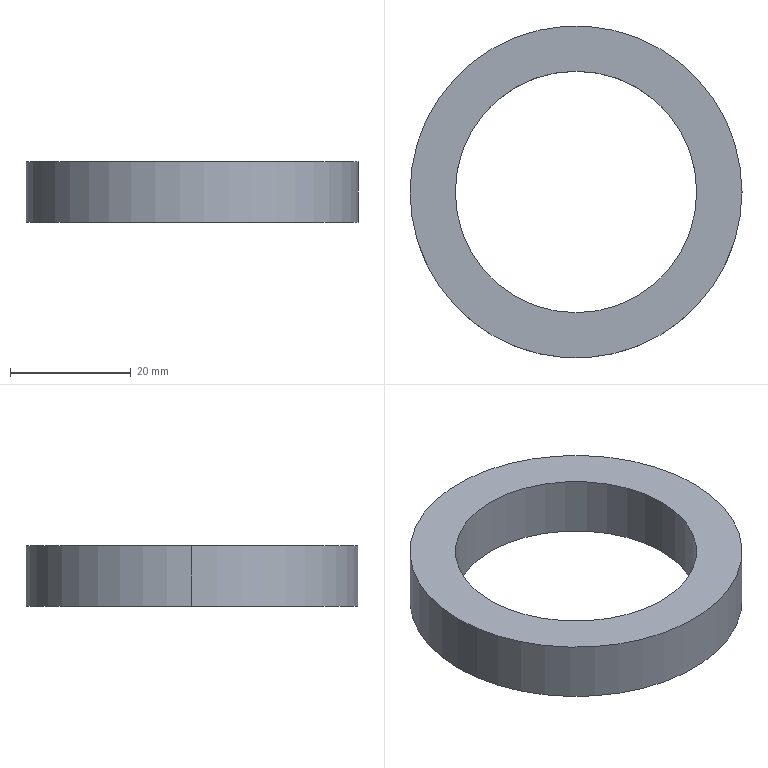Part | SolidWorks | features BaseBody 1 | 1 solid | 6 faces | box 55 x 55 x 10 mm | volume 11192 mm3 | cylinder 4 | plane 2 | commonest cylinder face diameters 40 x2 55 x2
STEP:
#1=CARTESIAN_POINT('',(27.5,0.,0.));
#2=VERTEX_POINT('',#1);
#3=CARTESIAN_POINT('',(-27.5,0.,0.));
#4=VERTEX_POINT('',#3);
#5=CARTESIAN_POINT('',(0.,0.,0.));
#6=DIRECTION('',(0.,0.,1.));
#7=DIRECTION('',(1.,0.,0.));
#8=AXIS2_PLACEMENT_3D('',#5,#6,#7);
#9=CIRCLE('',#8,27.5);
#10=EDGE_CURVE('',#2,#4,#9,.T.);
#11=ORIENTED_EDGE('',*,*,#10,.T.);
#12=CARTESIAN_POINT('',(-27.5,0.,10.));
#13=VERTEX_POINT('',#12);
#14=CARTESIAN_POINT('',(-27.5,0.,0.));
#15=DIRECTION('',(0.,0.,1.));
#16=VECTOR('',#15,1000.);
#17=LINE('',#14,#16);
#18=EDGE_CURVE('',#4,#13,#17,.T.);
#19=ORIENTED_EDGE('',*,*,#18,.T.);
#20=CARTESIAN_POINT('',(27.5,0.,10.));
#21=VERTEX_POINT('',#20);
#22=CARTESIAN_POINT('',(0.,0.,10.));
#23=DIRECTION('',(0.,0.,-1.));
#24=DIRECTION('',(1.,0.,0.));
#25=AXIS2_PLACEMENT_3D('',#22,#23,#24);
#26=CIRCLE('',#25,27.5);
#27=EDGE_CURVE('',#13,#21,#26,.T.);
#28=ORIENTED_EDGE('',*,*,#27,.T.);
#29=CARTESIAN_POINT('',(27.5,0.,0.));
#30=DIRECTION('',(0.,0.,1.));
#31=VECTOR('',#30,1000.);
#32=LINE('',#29,#31);
#33=EDGE_CURVE('',#2,#21,#32,.T.);
#34=ORIENTED_EDGE('',*,*,#33,.F.);
#35=EDGE_LOOP('',(#11,#19,#28,#34));
#36=FACE_OUTER_BOUND('',#35,.T.);
#37=CARTESIAN_POINT('',(0.,0.,0.));
#38=DIRECTION('',(0.,0.,1.));
#39=DIRECTION('',(1.,0.,0.));
#40=AXIS2_PLACEMENT_3D('',#37,#38,#39);
#41=CYLINDRICAL_SURFACE('',#40,27.5);
#42=ADVANCED_FACE('',(#36),#41,.T.);
#43=CARTESIAN_POINT('',(20.,0.,0.));
#44=VERTEX_POINT('',#43);
#45=CARTESIAN_POINT('',(-20.,0.,0.));
#46=VERTEX_POINT('',#45);
#47=CARTESIAN_POINT('',(0.,0.,0.));
#48=DIRECTION('',(0.,0.,-1.));
#49=DIRECTION('',(1.,0.,0.));
#50=AXIS2_PLACEMENT_3D('',#47,#48,#49);
#51=CIRCLE('',#50,20.);
#52=EDGE_CURVE('',#44,#46,#51,.T.);
#53=ORIENTED_EDGE('',*,*,#52,.T.);
#54=CARTESIAN_POINT('',(-20.,0.,10.));
#55=VERTEX_POINT('',#54);
#56=CARTESIAN_POINT('',(-20.,0.,0.));
#57=DIRECTION('',(0.,0.,1.));
#58=VECTOR('',#57,1000.);
#59=LINE('',#56,#58);
#60=EDGE_CURVE('',#46,#55,#59,.T.);
#61=ORIENTED_EDGE('',*,*,#60,.T.);
#62=CARTESIAN_POINT('',(20.,0.,10.));
#63=VERTEX_POINT('',#62);
#64=CARTESIAN_POINT('',(0.,0.,10.));
#65=DIRECTION('',(0.,0.,-1.));
#66=DIRECTION('',(1.,0.,0.));
#67=AXIS2_PLACEMENT_3D('',#64,#65,#66);
#68=CIRCLE('',#67,20.);
#69=EDGE_CURVE('',#63,#55,#68,.T.);
#70=ORIENTED_EDGE('',*,*,#69,.F.);
#71=CARTESIAN_POINT('',(20.,0.,0.));
#72=DIRECTION('',(0.,0.,1.));
#73=VECTOR('',#72,1000.);
#74=LINE('',#71,#73);
#75=EDGE_CURVE('',#44,#63,#74,.T.);
#76=ORIENTED_EDGE('',*,*,#75,.F.);
#77=EDGE_LOOP('',(#53,#61,#70,#76));
#78=FACE_OUTER_BOUND('',#77,.T.);
#79=CARTESIAN_POINT('',(0.,0.,0.));
#80=DIRECTION('',(0.,0.,1.));
#81=DIRECTION('',(1.,0.,0.));
#82=AXIS2_PLACEMENT_3D('',#79,#80,#81);
#83=CYLINDRICAL_SURFACE('',#82,20.);
#84=ADVANCED_FACE('',(#78),#83,.F.);
#85=ORIENTED_EDGE('',*,*,#18,.F.);
#86=CARTESIAN_POINT('',(0.,0.,0.));
#87=DIRECTION('',(0.,0.,1.));
#88=DIRECTION('',(1.,0.,0.));
#89=AXIS2_PLACEMENT_3D('',#86,#87,#88);
#90=CIRCLE('',#89,27.5);
#91=EDGE_CURVE('',#4,#2,#90,.T.);
#92=ORIENTED_EDGE('',*,*,#91,.T.);
#93=ORIENTED_EDGE('',*,*,#33,.T.);
#94=CARTESIAN_POINT('',(0.,0.,10.));
#95=DIRECTION('',(0.,0.,-1.));
#96=DIRECTION('',(1.,0.,0.));
#97=AXIS2_PLACEMENT_3D('',#94,#95,#96);
#98=CIRCLE('',#97,27.5);
#99=EDGE_CURVE('',#21,#13,#98,.T.);
#100=ORIENTED_EDGE('',*,*,#99,.T.);
#101=EDGE_LOOP('',(#85,#92,#93,#100));
#102=FACE_OUTER_BOUND('',#101,.T.);
#103=CARTESIAN_POINT('',(0.,0.,0.));
#104=DIRECTION('',(0.,0.,1.));
#105=DIRECTION('',(1.,0.,0.));
#106=AXIS2_PLACEMENT_3D('',#103,#104,#105);
#107=CYLINDRICAL_SURFACE('',#106,27.5);
#108=ADVANCED_FACE('',(#102),#107,.T.);
#109=ORIENTED_EDGE('',*,*,#52,.F.);
#110=CARTESIAN_POINT('',(0.,0.,0.));
#111=DIRECTION('',(0.,0.,-1.));
#112=DIRECTION('',(1.,0.,0.));
#113=AXIS2_PLACEMENT_3D('',#110,#111,#112);
#114=CIRCLE('',#113,20.);
#115=EDGE_CURVE('',#46,#44,#114,.T.);
#116=ORIENTED_EDGE('',*,*,#115,.F.);
#117=EDGE_LOOP('',(#109,#116));
#118=FACE_BOUND('',#117,.T.);
#119=ORIENTED_EDGE('',*,*,#10,.F.);
#120=ORIENTED_EDGE('',*,*,#91,.F.);
#121=EDGE_LOOP('',(#119,#120));
#122=FACE_OUTER_BOUND('',#121,.T.);
#123=CARTESIAN_POINT('',(0.,0.,0.));
#124=DIRECTION('',(0.,0.,1.));
#125=DIRECTION('',(1.,0.,0.));
#126=AXIS2_PLACEMENT_3D('',#123,#124,#125);
#127=PLANE('',#126);
#128=ADVANCED_FACE('',(#118,#122),#127,.F.);
#129=ORIENTED_EDGE('',*,*,#69,.T.);
#130=CARTESIAN_POINT('',(0.,0.,10.));
#131=DIRECTION('',(0.,0.,-1.));
#132=DIRECTION('',(1.,0.,0.));
#133=AXIS2_PLACEMENT_3D('',#130,#131,#132);
#134=CIRCLE('',#133,20.);
#135=EDGE_CURVE('',#55,#63,#134,.T.);
#136=ORIENTED_EDGE('',*,*,#135,.T.);
#137=EDGE_LOOP('',(#129,#136));
#138=FACE_BOUND('',#137,.T.);
#139=ORIENTED_EDGE('',*,*,#99,.F.);
#140=ORIENTED_EDGE('',*,*,#27,.F.);
#141=EDGE_LOOP('',(#139,#140));
#142=FACE_OUTER_BOUND('',#141,.T.);
#143=CARTESIAN_POINT('',(0.,0.,10.));
#144=DIRECTION('',(0.,0.,1.));
#145=DIRECTION('',(1.,0.,0.));
#146=AXIS2_PLACEMENT_3D('',#143,#144,#145);
#147=PLANE('',#146);
#148=ADVANCED_FACE('',(#138,#142),#147,.T.);
#149=ORIENTED_EDGE('',*,*,#60,.F.);
#150=ORIENTED_EDGE('',*,*,#115,.T.);
#151=ORIENTED_EDGE('',*,*,#75,.T.);
#152=ORIENTED_EDGE('',*,*,#135,.F.);
#153=EDGE_LOOP('',(#149,#150,#151,#152));
#154=FACE_OUTER_BOUND('',#153,.T.);
#155=CARTESIAN_POINT('',(0.,0.,0.));
#156=DIRECTION('',(0.,0.,1.));
#157=DIRECTION('',(1.,0.,0.));
#158=AXIS2_PLACEMENT_3D('',#155,#156,#157);
#159=CYLINDRICAL_SURFACE('',#158,20.);
#160=ADVANCED_FACE('',(#154),#159,.F.);
#161=CLOSED_SHELL('',(#42,#84,#108,#128,#148,#160));
#162=MANIFOLD_SOLID_BREP('',#161);
#163=CARTESIAN_POINT('',(0.,0.,0.));
#164=DIRECTION('',(0.,0.,1.));
#165=DIRECTION('',(1.,0.,0.));
#166=AXIS2_PLACEMENT_3D('',#163,#164,#165);
#167=(LENGTH_UNIT()NAMED_UNIT(*)SI_UNIT(.MILLI.,.METRE.));
#168=UNCERTAINTY_MEASURE_WITH_UNIT(LENGTH_MEASURE(0.00001),#167,'','');
#169=(NAMED_UNIT(*)PLANE_ANGLE_UNIT()SI_UNIT($,.RADIAN.));
#170=(NAMED_UNIT(*)SI_UNIT($,.STERADIAN.)SOLID_ANGLE_UNIT());
#171=(GEOMETRIC_REPRESENTATION_CONTEXT(3)GLOBAL_UNCERTAINTY_ASSIGNED_CONTEXT((#168))GLOBAL_UNIT_ASSIGNED_CONTEXT((#167,#169,#170))REPRESENTATION_CONTEXT('',''));
#172=ADVANCED_BREP_SHAPE_REPRESENTATION('',(#162,#166),#171);